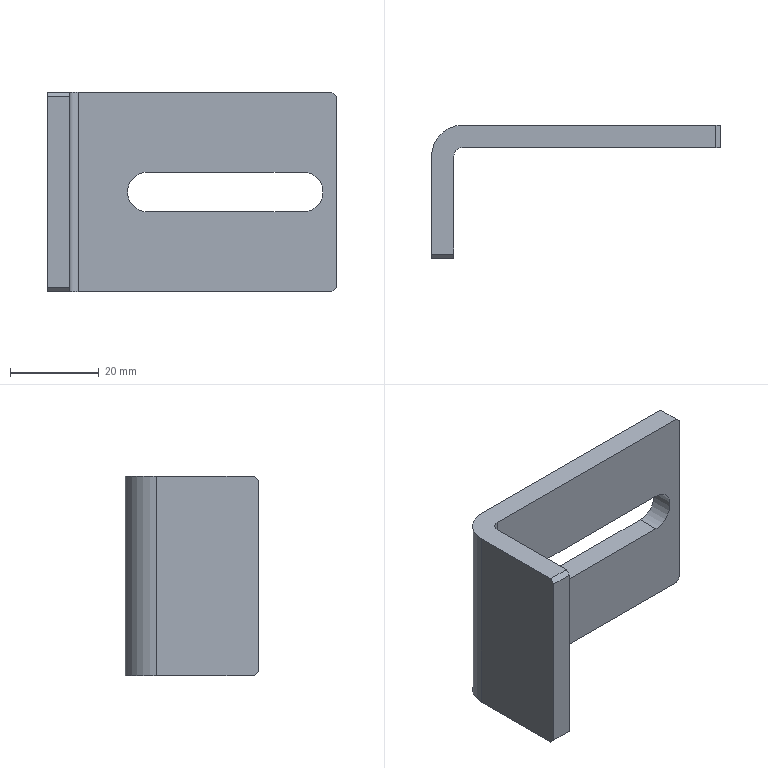Part | SolidWorks | features Fillet 2, Chamfer 1, ExtruThin 1, ICE 1 | 1 solid | 18 faces | box 65 x 30 x 45 mm | volume 17912 mm3 | plane 14 | cylinder 4 | commonest cylinder face diameters 9 x2 4 x1 14 x1
STEP:
#1=CARTESIAN_POINT('',(57.5,25.,18.));
#2=VERTEX_POINT('',#1);
#3=CARTESIAN_POINT('',(22.5,25.,18.));
#4=VERTEX_POINT('',#3);
#5=CARTESIAN_POINT('',(0.,25.,18.));
#6=DIRECTION('',(-1.,0.,0.));
#7=VECTOR('',#6,1000.);
#8=LINE('',#5,#7);
#9=EDGE_CURVE('',#2,#4,#8,.T.);
#10=ORIENTED_EDGE('',*,*,#9,.T.);
#11=CARTESIAN_POINT('',(22.5,25.,27.));
#12=VERTEX_POINT('',#11);
#13=CARTESIAN_POINT('',(22.5,25.,22.5));
#14=DIRECTION('',(0.,1.,0.));
#15=DIRECTION('',(0.,0.,1.));
#16=AXIS2_PLACEMENT_3D('',#13,#14,#15);
#17=CIRCLE('',#16,4.5);
#18=EDGE_CURVE('',#4,#12,#17,.T.);
#19=ORIENTED_EDGE('',*,*,#18,.T.);
#20=CARTESIAN_POINT('',(57.5,25.,27.));
#21=VERTEX_POINT('',#20);
#22=CARTESIAN_POINT('',(0.,25.,27.));
#23=DIRECTION('',(1.,0.,0.));
#24=VECTOR('',#23,1000.);
#25=LINE('',#22,#24);
#26=EDGE_CURVE('',#12,#21,#25,.T.);
#27=ORIENTED_EDGE('',*,*,#26,.T.);
#28=CARTESIAN_POINT('',(57.5,25.,22.5));
#29=DIRECTION('',(0.,1.,0.));
#30=DIRECTION('',(0.,0.,1.));
#31=AXIS2_PLACEMENT_3D('',#28,#29,#30);
#32=CIRCLE('',#31,4.5);
#33=EDGE_CURVE('',#21,#2,#32,.T.);
#34=ORIENTED_EDGE('',*,*,#33,.T.);
#35=EDGE_LOOP('',(#10,#19,#27,#34));
#36=FACE_BOUND('',#35,.T.);
#37=CARTESIAN_POINT('',(7.,25.,0.));
#38=VERTEX_POINT('',#37);
#39=CARTESIAN_POINT('',(64.,25.,0.));
#40=VERTEX_POINT('',#39);
#41=CARTESIAN_POINT('',(0.,25.,0.));
#42=DIRECTION('',(1.,0.,0.));
#43=VECTOR('',#42,1000.);
#44=LINE('',#41,#43);
#45=EDGE_CURVE('',#38,#40,#44,.T.);
#46=ORIENTED_EDGE('',*,*,#45,.T.);
#47=CARTESIAN_POINT('',(65.,25.,1.));
#48=VERTEX_POINT('',#47);
#49=CARTESIAN_POINT('',(64.,25.,0.));
#50=DIRECTION('',(0.7071,0.,0.7071));
#51=VECTOR('',#50,1000.);
#52=LINE('',#49,#51);
#53=EDGE_CURVE('',#40,#48,#52,.T.);
#54=ORIENTED_EDGE('',*,*,#53,.T.);
#55=CARTESIAN_POINT('',(65.,25.,44.));
#56=VERTEX_POINT('',#55);
#57=CARTESIAN_POINT('',(65.,25.,45.));
#58=DIRECTION('',(0.,0.,-1.));
#59=VECTOR('',#58,1000.);
#60=LINE('',#57,#59);
#61=EDGE_CURVE('',#56,#48,#60,.T.);
#62=ORIENTED_EDGE('',*,*,#61,.F.);
#63=CARTESIAN_POINT('',(64.,25.,45.));
#64=VERTEX_POINT('',#63);
#65=CARTESIAN_POINT('',(65.,25.,44.));
#66=DIRECTION('',(-0.7071,0.,0.7071));
#67=VECTOR('',#66,1000.);
#68=LINE('',#65,#67);
#69=EDGE_CURVE('',#56,#64,#68,.T.);
#70=ORIENTED_EDGE('',*,*,#69,.T.);
#71=CARTESIAN_POINT('',(7.,25.,45.));
#72=VERTEX_POINT('',#71);
#73=CARTESIAN_POINT('',(0.,25.,45.));
#74=DIRECTION('',(1.,0.,0.));
#75=VECTOR('',#74,1000.);
#76=LINE('',#73,#75);
#77=EDGE_CURVE('',#72,#64,#76,.T.);
#78=ORIENTED_EDGE('',*,*,#77,.F.);
#79=CARTESIAN_POINT('',(7.,25.,0.));
#80=DIRECTION('',(0.,0.,-1.));
#81=VECTOR('',#80,1000.);
#82=LINE('',#79,#81);
#83=EDGE_CURVE('',#72,#38,#82,.T.);
#84=ORIENTED_EDGE('',*,*,#83,.T.);
#85=EDGE_LOOP('',(#46,#54,#62,#70,#78,#84));
#86=FACE_OUTER_BOUND('',#85,.T.);
#87=CARTESIAN_POINT('',(0.,25.,45.));
#88=DIRECTION('',(0.,1.,0.));
#89=DIRECTION('',(0.,0.,1.));
#90=AXIS2_PLACEMENT_3D('',#87,#88,#89);
#91=PLANE('',#90);
#92=ADVANCED_FACE('',(#36,#86),#91,.F.);
#93=ORIENTED_EDGE('',*,*,#61,.T.);
#94=CARTESIAN_POINT('',(65.,30.,1.));
#95=VERTEX_POINT('',#94);
#96=CARTESIAN_POINT('',(65.,30.,1.));
#97=DIRECTION('',(0.,1.,0.));
#98=VECTOR('',#97,1000.);
#99=LINE('',#96,#98);
#100=EDGE_CURVE('',#48,#95,#99,.T.);
#101=ORIENTED_EDGE('',*,*,#100,.T.);
#102=CARTESIAN_POINT('',(65.,30.,44.));
#103=VERTEX_POINT('',#102);
#104=CARTESIAN_POINT('',(65.,30.,45.));
#105=DIRECTION('',(0.,0.,-1.));
#106=VECTOR('',#105,1000.);
#107=LINE('',#104,#106);
#108=EDGE_CURVE('',#103,#95,#107,.T.);
#109=ORIENTED_EDGE('',*,*,#108,.F.);
#110=CARTESIAN_POINT('',(65.,25.,44.));
#111=DIRECTION('',(0.,-1.,0.));
#112=VECTOR('',#111,1000.);
#113=LINE('',#110,#112);
#114=EDGE_CURVE('',#103,#56,#113,.T.);
#115=ORIENTED_EDGE('',*,*,#114,.T.);
#116=EDGE_LOOP('',(#93,#101,#109,#115));
#117=FACE_OUTER_BOUND('',#116,.T.);
#118=CARTESIAN_POINT('',(65.,30.,45.));
#119=DIRECTION('',(1.,0.,0.));
#120=DIRECTION('',(0.,0.,-1.));
#121=AXIS2_PLACEMENT_3D('',#118,#119,#120);
#122=PLANE('',#121);
#123=ADVANCED_FACE('',(#117),#122,.T.);
#124=CARTESIAN_POINT('',(22.5,30.,18.));
#125=VERTEX_POINT('',#124);
#126=CARTESIAN_POINT('',(22.5,30.,27.));
#127=VERTEX_POINT('',#126);
#128=CARTESIAN_POINT('',(22.5,30.,22.5));
#129=DIRECTION('',(0.,1.,0.));
#130=DIRECTION('',(0.,0.,1.));
#131=AXIS2_PLACEMENT_3D('',#128,#129,#130);
#132=CIRCLE('',#131,4.5);
#133=EDGE_CURVE('',#125,#127,#132,.T.);
#134=ORIENTED_EDGE('',*,*,#133,.F.);
#135=CARTESIAN_POINT('',(57.5,30.,18.));
#136=VERTEX_POINT('',#135);
#137=CARTESIAN_POINT('',(22.5,30.,18.));
#138=DIRECTION('',(-1.,0.,0.));
#139=VECTOR('',#138,1000.);
#140=LINE('',#137,#139);
#141=EDGE_CURVE('',#136,#125,#140,.T.);
#142=ORIENTED_EDGE('',*,*,#141,.F.);
#143=CARTESIAN_POINT('',(57.5,30.,27.));
#144=VERTEX_POINT('',#143);
#145=CARTESIAN_POINT('',(57.5,30.,22.5));
#146=DIRECTION('',(0.,1.,0.));
#147=DIRECTION('',(0.,0.,1.));
#148=AXIS2_PLACEMENT_3D('',#145,#146,#147);
#149=CIRCLE('',#148,4.5);
#150=EDGE_CURVE('',#144,#136,#149,.T.);
#151=ORIENTED_EDGE('',*,*,#150,.F.);
#152=CARTESIAN_POINT('',(22.5,30.,27.));
#153=DIRECTION('',(1.,0.,0.));
#154=VECTOR('',#153,1000.);
#155=LINE('',#152,#154);
#156=EDGE_CURVE('',#127,#144,#155,.T.);
#157=ORIENTED_EDGE('',*,*,#156,.F.);
#158=EDGE_LOOP('',(#134,#142,#151,#157));
#159=FACE_BOUND('',#158,.T.);
#160=ORIENTED_EDGE('',*,*,#108,.T.);
#161=CARTESIAN_POINT('',(64.,30.,0.));
#162=VERTEX_POINT('',#161);
#163=CARTESIAN_POINT('',(54.5,30.,-9.5));
#164=DIRECTION('',(-0.7071,0.,-0.7071));
#165=VECTOR('',#164,1000.);
#166=LINE('',#163,#165);
#167=EDGE_CURVE('',#95,#162,#166,.T.);
#168=ORIENTED_EDGE('',*,*,#167,.T.);
#169=CARTESIAN_POINT('',(7.,30.,0.));
#170=VERTEX_POINT('',#169);
#171=CARTESIAN_POINT('',(0.,30.,0.));
#172=DIRECTION('',(1.,0.,0.));
#173=VECTOR('',#172,1000.);
#174=LINE('',#171,#173);
#175=EDGE_CURVE('',#170,#162,#174,.T.);
#176=ORIENTED_EDGE('',*,*,#175,.F.);
#177=CARTESIAN_POINT('',(7.,30.,45.));
#178=VERTEX_POINT('',#177);
#179=CARTESIAN_POINT('',(7.,30.,45.));
#180=DIRECTION('',(0.,0.,1.));
#181=VECTOR('',#180,1000.);
#182=LINE('',#179,#181);
#183=EDGE_CURVE('',#170,#178,#182,.T.);
#184=ORIENTED_EDGE('',*,*,#183,.T.);
#185=CARTESIAN_POINT('',(64.,30.,45.));
#186=VERTEX_POINT('',#185);
#187=CARTESIAN_POINT('',(0.,30.,45.));
#188=DIRECTION('',(1.,0.,0.));
#189=VECTOR('',#188,1000.);
#190=LINE('',#187,#189);
#191=EDGE_CURVE('',#178,#186,#190,.T.);
#192=ORIENTED_EDGE('',*,*,#191,.T.);
#193=CARTESIAN_POINT('',(32.,30.,77.));
#194=DIRECTION('',(0.7071,0.,-0.7071));
#195=VECTOR('',#194,1000.);
#196=LINE('',#193,#195);
#197=EDGE_CURVE('',#186,#103,#196,.T.);
#198=ORIENTED_EDGE('',*,*,#197,.T.);
#199=EDGE_LOOP('',(#160,#168,#176,#184,#192,#198));
#200=FACE_OUTER_BOUND('',#199,.T.);
#201=CARTESIAN_POINT('',(0.,30.,45.));
#202=DIRECTION('',(0.,1.,0.));
#203=DIRECTION('',(0.,0.,1.));
#204=AXIS2_PLACEMENT_3D('',#201,#202,#203);
#205=PLANE('',#204);
#206=ADVANCED_FACE('',(#159,#200),#205,.T.);
#207=CARTESIAN_POINT('',(0.,1.,0.));
#208=VERTEX_POINT('',#207);
#209=CARTESIAN_POINT('',(0.,23.,0.));
#210=VERTEX_POINT('',#209);
#211=CARTESIAN_POINT('',(0.,0.,0.));
#212=DIRECTION('',(0.,1.,0.));
#213=VECTOR('',#212,1000.);
#214=LINE('',#211,#213);
#215=EDGE_CURVE('',#208,#210,#214,.T.);
#216=ORIENTED_EDGE('',*,*,#215,.F.);
#217=CARTESIAN_POINT('',(0.,0.,1.));
#218=VERTEX_POINT('',#217);
#219=CARTESIAN_POINT('',(0.,-22.,23.));
#220=DIRECTION('',(0.,-0.7071,0.7071));
#221=VECTOR('',#220,1000.);
#222=LINE('',#219,#221);
#223=EDGE_CURVE('',#208,#218,#222,.T.);
#224=ORIENTED_EDGE('',*,*,#223,.T.);
#225=CARTESIAN_POINT('',(0.,0.,44.));
#226=VERTEX_POINT('',#225);
#227=CARTESIAN_POINT('',(0.,0.,45.));
#228=DIRECTION('',(0.,0.,-1.));
#229=VECTOR('',#228,1000.);
#230=LINE('',#227,#229);
#231=EDGE_CURVE('',#226,#218,#230,.T.);
#232=ORIENTED_EDGE('',*,*,#231,.F.);
#233=CARTESIAN_POINT('',(0.,1.,45.));
#234=VERTEX_POINT('',#233);
#235=CARTESIAN_POINT('',(0.,0.5,44.5));
#236=DIRECTION('',(0.,0.7071,0.7071));
#237=VECTOR('',#236,1000.);
#238=LINE('',#235,#237);
#239=EDGE_CURVE('',#226,#234,#238,.T.);
#240=ORIENTED_EDGE('',*,*,#239,.T.);
#241=CARTESIAN_POINT('',(0.,23.,45.));
#242=VERTEX_POINT('',#241);
#243=CARTESIAN_POINT('',(0.,0.,45.));
#244=DIRECTION('',(0.,1.,0.));
#245=VECTOR('',#244,1000.);
#246=LINE('',#243,#245);
#247=EDGE_CURVE('',#234,#242,#246,.T.);
#248=ORIENTED_EDGE('',*,*,#247,.T.);
#249=CARTESIAN_POINT('',(0.,23.,45.));
#250=DIRECTION('',(0.,0.,-1.));
#251=VECTOR('',#250,1000.);
#252=LINE('',#249,#251);
#253=EDGE_CURVE('',#242,#210,#252,.T.);
#254=ORIENTED_EDGE('',*,*,#253,.T.);
#255=EDGE_LOOP('',(#216,#224,#232,#240,#248,#254));
#256=FACE_OUTER_BOUND('',#255,.T.);
#257=CARTESIAN_POINT('',(0.,0.,45.));
#258=DIRECTION('',(-1.,0.,0.));
#259=DIRECTION('',(0.,0.,1.));
#260=AXIS2_PLACEMENT_3D('',#257,#258,#259);
#261=PLANE('',#260);
#262=ADVANCED_FACE('',(#256),#261,.T.);
#263=ORIENTED_EDGE('',*,*,#231,.T.);
#264=CARTESIAN_POINT('',(5.,0.,1.));
#265=VERTEX_POINT('',#264);
#266=CARTESIAN_POINT('',(5.,0.,1.));
#267=DIRECTION('',(1.,0.,0.));
#268=VECTOR('',#267,1000.);
#269=LINE('',#266,#268);
#270=EDGE_CURVE('',#218,#265,#269,.T.);
#271=ORIENTED_EDGE('',*,*,#270,.T.);
#272=CARTESIAN_POINT('',(5.,0.,44.));
#273=VERTEX_POINT('',#272);
#274=CARTESIAN_POINT('',(5.,0.,45.));
#275=DIRECTION('',(0.,0.,-1.));
#276=VECTOR('',#275,1000.);
#277=LINE('',#274,#276);
#278=EDGE_CURVE('',#273,#265,#277,.T.);
#279=ORIENTED_EDGE('',*,*,#278,.F.);
#280=CARTESIAN_POINT('',(0.,0.,44.));
#281=DIRECTION('',(-1.,0.,0.));
#282=VECTOR('',#281,1000.);
#283=LINE('',#280,#282);
#284=EDGE_CURVE('',#273,#226,#283,.T.);
#285=ORIENTED_EDGE('',*,*,#284,.T.);
#286=EDGE_LOOP('',(#263,#271,#279,#285));
#287=FACE_OUTER_BOUND('',#286,.T.);
#288=CARTESIAN_POINT('',(5.,0.,45.));
#289=DIRECTION('',(0.,-1.,0.));
#290=DIRECTION('',(0.,0.,-1.));
#291=AXIS2_PLACEMENT_3D('',#288,#289,#290);
#292=PLANE('',#291);
#293=ADVANCED_FACE('',(#287),#292,.T.);
#294=ORIENTED_EDGE('',*,*,#278,.T.);
#295=CARTESIAN_POINT('',(5.,1.,0.));
#296=VERTEX_POINT('',#295);
#297=CARTESIAN_POINT('',(5.,1.,0.));
#298=DIRECTION('',(0.,0.7071,-0.7071));
#299=VECTOR('',#298,1000.);
#300=LINE('',#297,#299);
#301=EDGE_CURVE('',#265,#296,#300,.T.);
#302=ORIENTED_EDGE('',*,*,#301,.T.);
#303=CARTESIAN_POINT('',(5.,23.,0.));
#304=VERTEX_POINT('',#303);
#305=CARTESIAN_POINT('',(5.,0.,0.));
#306=DIRECTION('',(0.,1.,0.));
#307=VECTOR('',#306,1000.);
#308=LINE('',#305,#307);
#309=EDGE_CURVE('',#296,#304,#308,.T.);
#310=ORIENTED_EDGE('',*,*,#309,.T.);
#311=CARTESIAN_POINT('',(5.,23.,45.));
#312=VERTEX_POINT('',#311);
#313=CARTESIAN_POINT('',(5.,23.,45.));
#314=DIRECTION('',(0.,0.,1.));
#315=VECTOR('',#314,1000.);
#316=LINE('',#313,#315);
#317=EDGE_CURVE('',#304,#312,#316,.T.);
#318=ORIENTED_EDGE('',*,*,#317,.T.);
#319=CARTESIAN_POINT('',(5.,1.,45.));
#320=VERTEX_POINT('',#319);
#321=CARTESIAN_POINT('',(5.,0.,45.));
#322=DIRECTION('',(0.,1.,0.));
#323=VECTOR('',#322,1000.);
#324=LINE('',#321,#323);
#325=EDGE_CURVE('',#320,#312,#324,.T.);
#326=ORIENTED_EDGE('',*,*,#325,.F.);
#327=CARTESIAN_POINT('',(5.,0.,44.));
#328=DIRECTION('',(0.,-0.7071,-0.7071));
#329=VECTOR('',#328,1000.);
#330=LINE('',#327,#329);
#331=EDGE_CURVE('',#320,#273,#330,.T.);
#332=ORIENTED_EDGE('',*,*,#331,.T.);
#333=EDGE_LOOP('',(#294,#302,#310,#318,#326,#332));
#334=FACE_OUTER_BOUND('',#333,.T.);
#335=CARTESIAN_POINT('',(5.,0.,45.));
#336=DIRECTION('',(-1.,0.,0.));
#337=DIRECTION('',(0.,0.,1.));
#338=AXIS2_PLACEMENT_3D('',#335,#336,#337);
#339=PLANE('',#338);
#340=ADVANCED_FACE('',(#334),#339,.F.);
#341=ORIENTED_EDGE('',*,*,#247,.F.);
#342=CARTESIAN_POINT('',(5.,1.,45.));
#343=DIRECTION('',(1.,0.,0.));
#344=VECTOR('',#343,1000.);
#345=LINE('',#342,#344);
#346=EDGE_CURVE('',#234,#320,#345,.T.);
#347=ORIENTED_EDGE('',*,*,#346,.T.);
#348=ORIENTED_EDGE('',*,*,#325,.T.);
#349=CARTESIAN_POINT('',(7.,23.,45.));
#350=DIRECTION('',(0.,0.,-1.));
#351=DIRECTION('',(-1.,0.,0.));
#352=AXIS2_PLACEMENT_3D('',#349,#350,#351);
#353=CIRCLE('',#352,2.);
#354=EDGE_CURVE('',#312,#72,#353,.T.);
#355=ORIENTED_EDGE('',*,*,#354,.T.);
#356=ORIENTED_EDGE('',*,*,#77,.T.);
#357=CARTESIAN_POINT('',(64.,30.,45.));
#358=DIRECTION('',(0.,1.,0.));
#359=VECTOR('',#358,1000.);
#360=LINE('',#357,#359);
#361=EDGE_CURVE('',#64,#186,#360,.T.);
#362=ORIENTED_EDGE('',*,*,#361,.T.);
#363=ORIENTED_EDGE('',*,*,#191,.F.);
#364=CARTESIAN_POINT('',(7.,23.,45.));
#365=DIRECTION('',(0.,0.,1.));
#366=DIRECTION('',(-1.,0.,0.));
#367=AXIS2_PLACEMENT_3D('',#364,#365,#366);
#368=CIRCLE('',#367,7.);
#369=EDGE_CURVE('',#178,#242,#368,.T.);
#370=ORIENTED_EDGE('',*,*,#369,.T.);
#371=EDGE_LOOP('',(#341,#347,#348,#355,#356,#362,#363,#370));
#372=FACE_OUTER_BOUND('',#371,.T.);
#373=CARTESIAN_POINT('',(0.,0.,45.));
#374=DIRECTION('',(0.,0.,-1.));
#375=DIRECTION('',(-1.,0.,0.));
#376=AXIS2_PLACEMENT_3D('',#373,#374,#375);
#377=PLANE('',#376);
#378=ADVANCED_FACE('',(#372),#377,.F.);
#379=ORIENTED_EDGE('',*,*,#309,.F.);
#380=CARTESIAN_POINT('',(0.,1.,0.));
#381=DIRECTION('',(-1.,0.,0.));
#382=VECTOR('',#381,1000.);
#383=LINE('',#380,#382);
#384=EDGE_CURVE('',#296,#208,#383,.T.);
#385=ORIENTED_EDGE('',*,*,#384,.T.);
#386=ORIENTED_EDGE('',*,*,#215,.T.);
#387=CARTESIAN_POINT('',(7.,23.,0.));
#388=DIRECTION('',(0.,0.,-1.));
#389=DIRECTION('',(-1.,0.,0.));
#390=AXIS2_PLACEMENT_3D('',#387,#388,#389);
#391=CIRCLE('',#390,7.);
#392=EDGE_CURVE('',#210,#170,#391,.T.);
#393=ORIENTED_EDGE('',*,*,#392,.T.);
#394=ORIENTED_EDGE('',*,*,#175,.T.);
#395=CARTESIAN_POINT('',(64.,0.,0.));
#396=DIRECTION('',(0.,-1.,0.));
#397=VECTOR('',#396,1000.);
#398=LINE('',#395,#397);
#399=EDGE_CURVE('',#162,#40,#398,.T.);
#400=ORIENTED_EDGE('',*,*,#399,.T.);
#401=ORIENTED_EDGE('',*,*,#45,.F.);
#402=CARTESIAN_POINT('',(7.,23.,0.));
#403=DIRECTION('',(0.,0.,1.));
#404=DIRECTION('',(-1.,0.,0.));
#405=AXIS2_PLACEMENT_3D('',#402,#403,#404);
#406=CIRCLE('',#405,2.);
#407=EDGE_CURVE('',#38,#304,#406,.T.);
#408=ORIENTED_EDGE('',*,*,#407,.T.);
#409=EDGE_LOOP('',(#379,#385,#386,#393,#394,#400,#401,#408));
#410=FACE_OUTER_BOUND('',#409,.T.);
#411=CARTESIAN_POINT('',(0.,0.,0.));
#412=DIRECTION('',(0.,0.,-1.));
#413=DIRECTION('',(-1.,0.,0.));
#414=AXIS2_PLACEMENT_3D('',#411,#412,#413);
#415=PLANE('',#414);
#416=ADVANCED_FACE('',(#410),#415,.T.);
#417=ORIENTED_EDGE('',*,*,#354,.F.);
#418=ORIENTED_EDGE('',*,*,#317,.F.);
#419=ORIENTED_EDGE('',*,*,#407,.F.);
#420=ORIENTED_EDGE('',*,*,#83,.F.);
#421=EDGE_LOOP('',(#417,#418,#419,#420));
#422=FACE_OUTER_BOUND('',#421,.T.);
#423=CARTESIAN_POINT('',(7.,23.,45.));
#424=DIRECTION('',(0.,0.,1.));
#425=DIRECTION('',(1.,0.,0.));
#426=AXIS2_PLACEMENT_3D('',#423,#424,#425);
#427=CYLINDRICAL_SURFACE('',#426,2.);
#428=ADVANCED_FACE('',(#422),#427,.F.);
#429=ORIENTED_EDGE('',*,*,#369,.F.);
#430=ORIENTED_EDGE('',*,*,#183,.F.);
#431=ORIENTED_EDGE('',*,*,#392,.F.);
#432=ORIENTED_EDGE('',*,*,#253,.F.);
#433=EDGE_LOOP('',(#429,#430,#431,#432));
#434=FACE_OUTER_BOUND('',#433,.T.);
#435=CARTESIAN_POINT('',(7.,23.,45.));
#436=DIRECTION('',(0.,0.,-1.));
#437=DIRECTION('',(-1.,0.,0.));
#438=AXIS2_PLACEMENT_3D('',#435,#436,#437);
#439=CYLINDRICAL_SURFACE('',#438,7.);
#440=ADVANCED_FACE('',(#434),#439,.T.);
#441=ORIENTED_EDGE('',*,*,#301,.F.);
#442=ORIENTED_EDGE('',*,*,#270,.F.);
#443=ORIENTED_EDGE('',*,*,#223,.F.);
#444=ORIENTED_EDGE('',*,*,#384,.F.);
#445=EDGE_LOOP('',(#441,#442,#443,#444));
#446=FACE_OUTER_BOUND('',#445,.T.);
#447=CARTESIAN_POINT('',(0.,1.,0.));
#448=DIRECTION('',(0.,0.7071,0.7071));
#449=DIRECTION('',(-1.,0.,0.));
#450=AXIS2_PLACEMENT_3D('',#447,#448,#449);
#451=PLANE('',#450);
#452=ADVANCED_FACE('',(#446),#451,.F.);
#453=ORIENTED_EDGE('',*,*,#331,.F.);
#454=ORIENTED_EDGE('',*,*,#346,.F.);
#455=ORIENTED_EDGE('',*,*,#239,.F.);
#456=ORIENTED_EDGE('',*,*,#284,.F.);
#457=EDGE_LOOP('',(#453,#454,#455,#456));
#458=FACE_OUTER_BOUND('',#457,.T.);
#459=CARTESIAN_POINT('',(5.,0.,44.));
#460=DIRECTION('',(0.,-0.7071,0.7071));
#461=DIRECTION('',(1.,0.,0.));
#462=AXIS2_PLACEMENT_3D('',#459,#460,#461);
#463=PLANE('',#462);
#464=ADVANCED_FACE('',(#458),#463,.T.);
#465=ORIENTED_EDGE('',*,*,#167,.F.);
#466=ORIENTED_EDGE('',*,*,#100,.F.);
#467=ORIENTED_EDGE('',*,*,#53,.F.);
#468=ORIENTED_EDGE('',*,*,#399,.F.);
#469=EDGE_LOOP('',(#465,#466,#467,#468));
#470=FACE_OUTER_BOUND('',#469,.T.);
#471=CARTESIAN_POINT('',(64.,0.,0.));
#472=DIRECTION('',(-0.7071,0.,0.7071));
#473=DIRECTION('',(0.,-1.,0.));
#474=AXIS2_PLACEMENT_3D('',#471,#472,#473);
#475=PLANE('',#474);
#476=ADVANCED_FACE('',(#470),#475,.F.);
#477=ORIENTED_EDGE('',*,*,#197,.F.);
#478=ORIENTED_EDGE('',*,*,#361,.F.);
#479=ORIENTED_EDGE('',*,*,#69,.F.);
#480=ORIENTED_EDGE('',*,*,#114,.F.);
#481=EDGE_LOOP('',(#477,#478,#479,#480));
#482=FACE_OUTER_BOUND('',#481,.T.);
#483=CARTESIAN_POINT('',(65.,30.,44.));
#484=DIRECTION('',(0.7071,0.,0.7071));
#485=DIRECTION('',(0.,1.,0.));
#486=AXIS2_PLACEMENT_3D('',#483,#484,#485);
#487=PLANE('',#486);
#488=ADVANCED_FACE('',(#482),#487,.T.);
#489=CARTESIAN_POINT('',(22.5,0.,18.));
#490=DIRECTION('',(0.,1.,0.));
#491=VECTOR('',#490,1000.);
#492=LINE('',#489,#491);
#493=EDGE_CURVE('',#4,#125,#492,.T.);
#494=ORIENTED_EDGE('',*,*,#493,.T.);
#495=ORIENTED_EDGE('',*,*,#133,.T.);
#496=CARTESIAN_POINT('',(22.5,0.,27.));
#497=DIRECTION('',(0.,1.,0.));
#498=VECTOR('',#497,1000.);
#499=LINE('',#496,#498);
#500=EDGE_CURVE('',#12,#127,#499,.T.);
#501=ORIENTED_EDGE('',*,*,#500,.F.);
#502=ORIENTED_EDGE('',*,*,#18,.F.);
#503=EDGE_LOOP('',(#494,#495,#501,#502));
#504=FACE_OUTER_BOUND('',#503,.T.);
#505=CARTESIAN_POINT('',(22.5,0.,22.5));
#506=DIRECTION('',(0.,1.,0.));
#507=DIRECTION('',(0.,0.,1.));
#508=AXIS2_PLACEMENT_3D('',#505,#506,#507);
#509=CYLINDRICAL_SURFACE('',#508,4.5);
#510=ADVANCED_FACE('',(#504),#509,.F.);
#511=CARTESIAN_POINT('',(57.5,0.,18.));
#512=DIRECTION('',(0.,1.,0.));
#513=VECTOR('',#512,1000.);
#514=LINE('',#511,#513);
#515=EDGE_CURVE('',#2,#136,#514,.T.);
#516=ORIENTED_EDGE('',*,*,#515,.T.);
#517=ORIENTED_EDGE('',*,*,#141,.T.);
#518=ORIENTED_EDGE('',*,*,#493,.F.);
#519=ORIENTED_EDGE('',*,*,#9,.F.);
#520=EDGE_LOOP('',(#516,#517,#518,#519));
#521=FACE_OUTER_BOUND('',#520,.T.);
#522=CARTESIAN_POINT('',(22.5,0.,18.));
#523=DIRECTION('',(0.,0.,-1.));
#524=DIRECTION('',(-1.,0.,0.));
#525=AXIS2_PLACEMENT_3D('',#522,#523,#524);
#526=PLANE('',#525);
#527=ADVANCED_FACE('',(#521),#526,.F.);
#528=CARTESIAN_POINT('',(57.5,0.,27.));
#529=DIRECTION('',(0.,1.,0.));
#530=VECTOR('',#529,1000.);
#531=LINE('',#528,#530);
#532=EDGE_CURVE('',#21,#144,#531,.T.);
#533=ORIENTED_EDGE('',*,*,#532,.T.);
#534=ORIENTED_EDGE('',*,*,#150,.T.);
#535=ORIENTED_EDGE('',*,*,#515,.F.);
#536=ORIENTED_EDGE('',*,*,#33,.F.);
#537=EDGE_LOOP('',(#533,#534,#535,#536));
#538=FACE_OUTER_BOUND('',#537,.T.);
#539=CARTESIAN_POINT('',(57.5,0.,22.5));
#540=DIRECTION('',(0.,1.,0.));
#541=DIRECTION('',(0.,0.,1.));
#542=AXIS2_PLACEMENT_3D('',#539,#540,#541);
#543=CYLINDRICAL_SURFACE('',#542,4.5);
#544=ADVANCED_FACE('',(#538),#543,.F.);
#545=ORIENTED_EDGE('',*,*,#500,.T.);
#546=ORIENTED_EDGE('',*,*,#156,.T.);
#547=ORIENTED_EDGE('',*,*,#532,.F.);
#548=ORIENTED_EDGE('',*,*,#26,.F.);
#549=EDGE_LOOP('',(#545,#546,#547,#548));
#550=FACE_OUTER_BOUND('',#549,.T.);
#551=CARTESIAN_POINT('',(22.5,0.,27.));
#552=DIRECTION('',(0.,0.,1.));
#553=DIRECTION('',(1.,0.,0.));
#554=AXIS2_PLACEMENT_3D('',#551,#552,#553);
#555=PLANE('',#554);
#556=ADVANCED_FACE('',(#550),#555,.F.);
#557=CLOSED_SHELL('',(#92,#123,#206,#262,#293,#340,#378,#416,#428,#440,#452,#464,#476,#488,#510,#527,#544,#556));
#558=MANIFOLD_SOLID_BREP('',#557);
#559=CARTESIAN_POINT('',(0.,0.,0.));
#560=DIRECTION('',(0.,0.,1.));
#561=DIRECTION('',(1.,0.,0.));
#562=AXIS2_PLACEMENT_3D('',#559,#560,#561);
#563=(LENGTH_UNIT()NAMED_UNIT(*)SI_UNIT(.MILLI.,.METRE.));
#564=UNCERTAINTY_MEASURE_WITH_UNIT(LENGTH_MEASURE(0.00001),#563,'','');
#565=(NAMED_UNIT(*)PLANE_ANGLE_UNIT()SI_UNIT($,.RADIAN.));
#566=(NAMED_UNIT(*)SI_UNIT($,.STERADIAN.)SOLID_ANGLE_UNIT());
#567=(GEOMETRIC_REPRESENTATION_CONTEXT(3)GLOBAL_UNCERTAINTY_ASSIGNED_CONTEXT((#564))GLOBAL_UNIT_ASSIGNED_CONTEXT((#563,#565,#566))REPRESENTATION_CONTEXT('',''));
#568=ADVANCED_BREP_SHAPE_REPRESENTATION('',(#558,#562),#567);